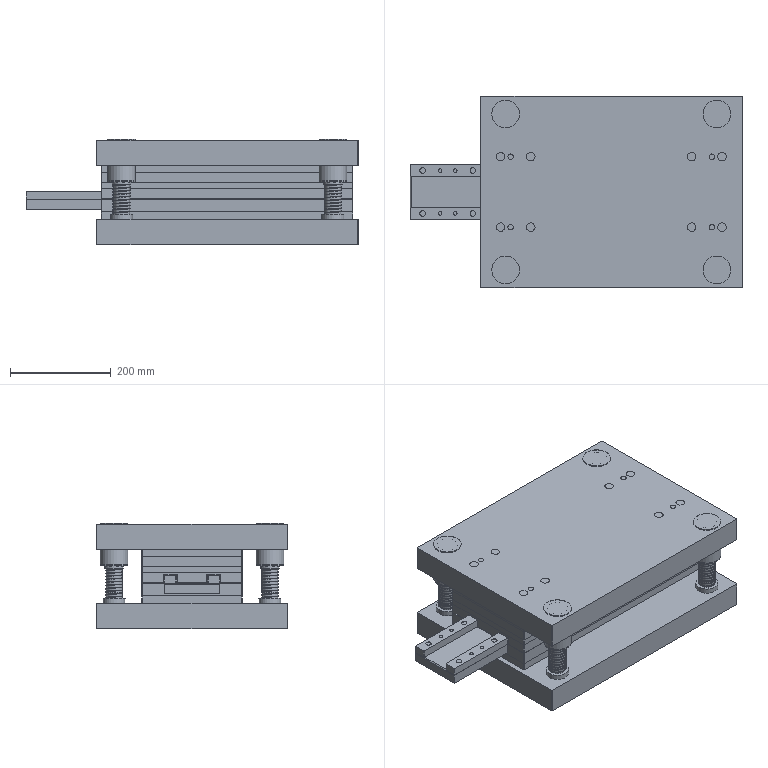Part | NX | features BREP 280 | 432 solids | 6809 faces | volume 34244157 mm3 | plane 3841 | cylinder 2136 | sphere 648 | cone 100 | torus 76 | spline 8 | commonest cylinder face diameters 1 x570 1.1 x224 0.9 x153 10 x88 3.1 x70 1.05 x65